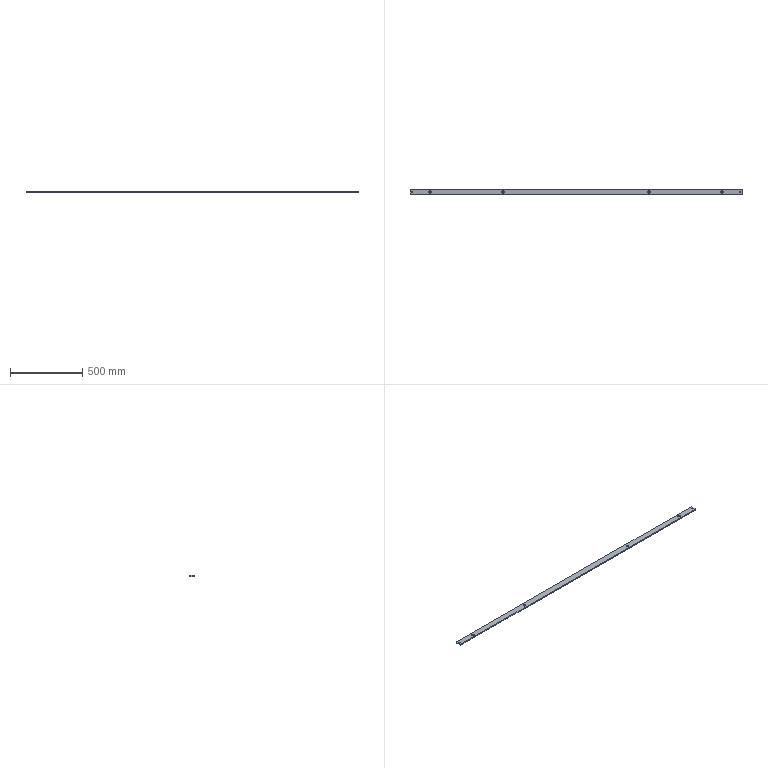Part | STEP file | rectangular profile 40x8-2303 | 1 solid | 20 faces | box 2303 x 40 x 8 mm | volume 732827 mm3 | spline 10 | plane 10